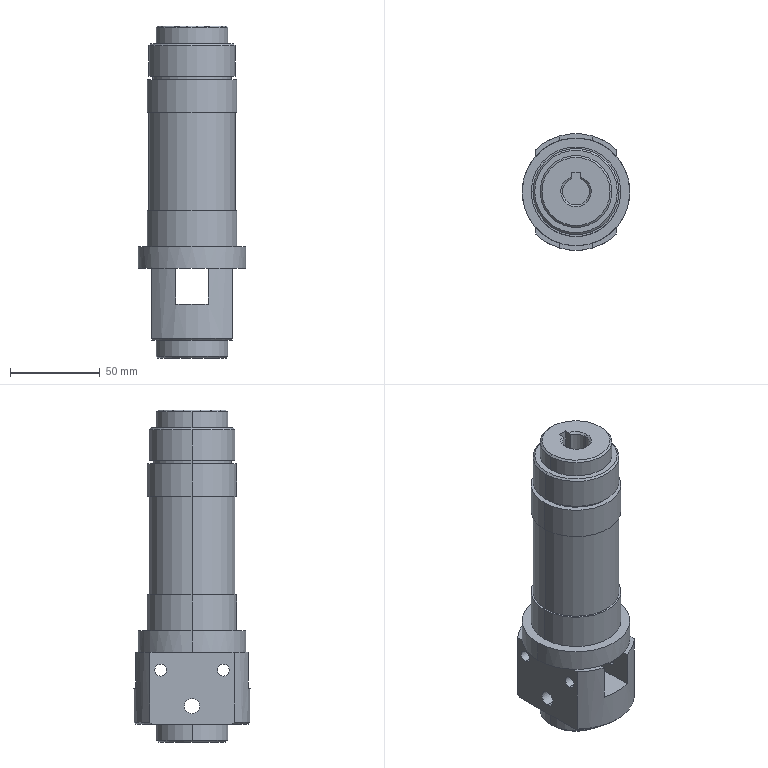Part | STEP file | YCD14007A-08.03.08.01 Shaft (Cylinder) | 1 solid | 70 faces | box 60 x 65 x 185 mm | volume 338320 mm3 | cylinder 33 | plane 26 | cone 11 | commonest cylinder face diameters 6.6 x8 40 x4 48 x4 50 x4 15 x3 8.5 x2